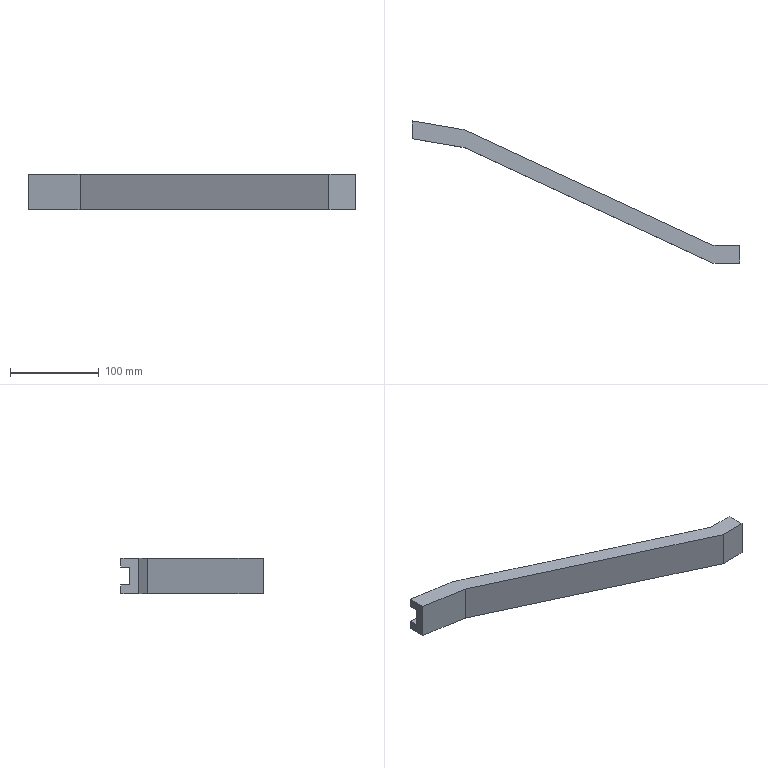Part | STEP file | Part2_4 | 1 solid | 22 faces | box 368.104 x 160 x 40 mm | volume 215115 mm3 | plane 20 | cylinder 2 | commonest cylinder face diameters 20 x2